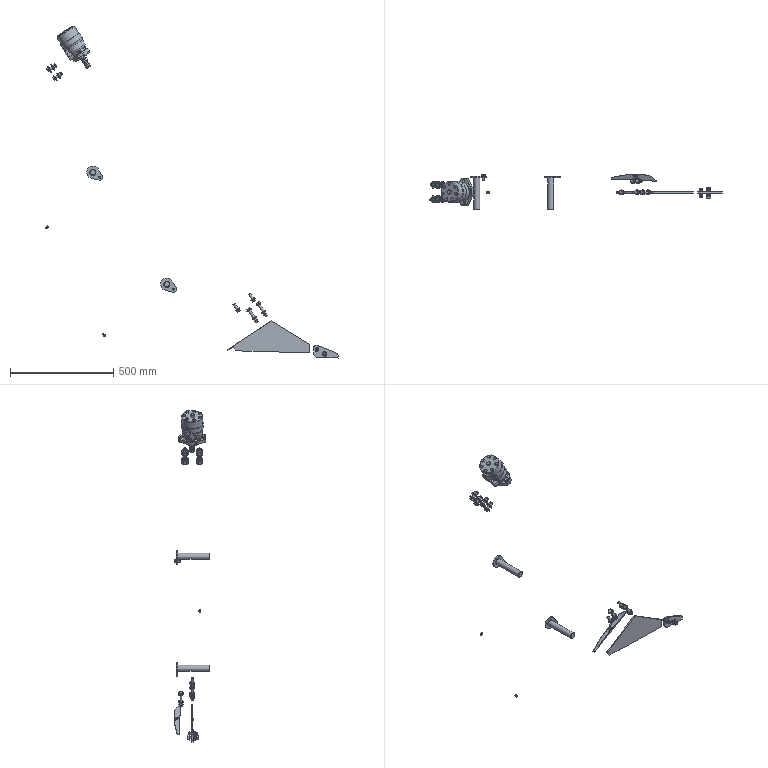Part | STEP file | COMPOUND | 60 solids | 878 faces | box 1417 x 170.85 x 1608 mm | volume 1769847 mm3 | plane 511 | cylinder 165 | cone 146 | other 28 | torus 20 | spline 6 | sphere 2 | commonest cylinder face diameters 12 x16 13 x15 10 x13 24 x9 12.55 x8 18.75 x8